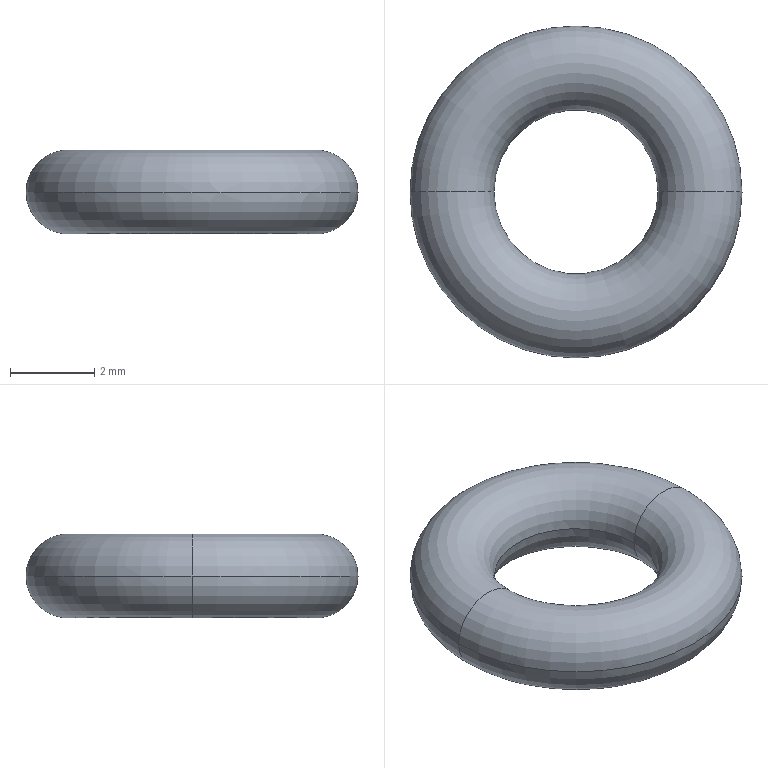Part | STEP file | ZXW722-L-79-3 | 1 solid | 4 faces | box 7.9 x 7.9 x 2 mm | volume 58.231 mm3 | torus 4
STEP:
#1=CARTESIAN_POINT('',(0.,0.,0.));
#2=DIRECTION('',(0.,0.,1.));
#3=DIRECTION('',(1.,0.,0.));
#4=AXIS2_PLACEMENT_3D('',#1,#2,#3);
#5=CARTESIAN_POINT('',(1.95,0.,-1.));
#6=VERTEX_POINT('',#5);
#7=CARTESIAN_POINT('',(3.95,0.,-1.));
#8=VERTEX_POINT('',#7);
#9=CARTESIAN_POINT('',(2.95,0.,-1.));
#10=DIRECTION('',(0.,-1.,0.));
#11=DIRECTION('',(-1.,0.,0.));
#12=AXIS2_PLACEMENT_3D('',#9,#10,#11);
#13=CIRCLE('',#12,1.);
#14=EDGE_CURVE('',#6,#8,#13,.T.);
#15=ORIENTED_EDGE('',*,*,#14,.T.);
#16=CARTESIAN_POINT('',(-3.95,0.,-1.));
#17=VERTEX_POINT('',#16);
#18=CARTESIAN_POINT('',(0.,0.,-1.));
#19=DIRECTION('',(0.,0.,-1.));
#20=DIRECTION('',(-1.,0.,0.));
#21=AXIS2_PLACEMENT_3D('',#18,#19,#20);
#22=CIRCLE('',#21,3.95);
#23=EDGE_CURVE('',#17,#8,#22,.T.);
#24=ORIENTED_EDGE('',*,*,#23,.F.);
#25=CARTESIAN_POINT('',(-1.95,0.,-1.));
#26=VERTEX_POINT('',#25);
#27=CARTESIAN_POINT('',(-2.95,0.,-1.));
#28=DIRECTION('',(0.,1.,0.));
#29=DIRECTION('',(1.,0.,0.));
#30=AXIS2_PLACEMENT_3D('',#27,#28,#29);
#31=CIRCLE('',#30,1.);
#32=EDGE_CURVE('',#26,#17,#31,.T.);
#33=ORIENTED_EDGE('',*,*,#32,.F.);
#34=CARTESIAN_POINT('',(0.,0.,-1.));
#35=DIRECTION('',(0.,0.,-1.));
#36=DIRECTION('',(-1.,0.,0.));
#37=AXIS2_PLACEMENT_3D('',#34,#35,#36);
#38=CIRCLE('',#37,1.95);
#39=EDGE_CURVE('',#26,#6,#38,.T.);
#40=ORIENTED_EDGE('',*,*,#39,.T.);
#41=EDGE_LOOP('',(#15,#24,#33,#40));
#42=FACE_OUTER_BOUND('',#41,.F.);
#43=CARTESIAN_POINT('',(0.,0.,-1.));
#44=DIRECTION('',(0.,0.,1.));
#45=DIRECTION('',(-1.,0.,0.));
#46=AXIS2_PLACEMENT_3D('',#43,#44,#45);
#47=TOROIDAL_SURFACE('',#46,2.95,1.);
#48=ADVANCED_FACE('',(#42),#47,.T.);
#49=ORIENTED_EDGE('',*,*,#14,.F.);
#50=CARTESIAN_POINT('',(0.,0.,-1.));
#51=DIRECTION('',(0.,0.,1.));
#52=DIRECTION('',(-1.,0.,0.));
#53=AXIS2_PLACEMENT_3D('',#50,#51,#52);
#54=CIRCLE('',#53,1.95);
#55=EDGE_CURVE('',#26,#6,#54,.T.);
#56=ORIENTED_EDGE('',*,*,#55,.F.);
#57=ORIENTED_EDGE('',*,*,#32,.T.);
#58=CARTESIAN_POINT('',(0.,0.,-1.));
#59=DIRECTION('',(0.,0.,1.));
#60=DIRECTION('',(-1.,0.,0.));
#61=AXIS2_PLACEMENT_3D('',#58,#59,#60);
#62=CIRCLE('',#61,3.95);
#63=EDGE_CURVE('',#17,#8,#62,.T.);
#64=ORIENTED_EDGE('',*,*,#63,.T.);
#65=EDGE_LOOP('',(#49,#56,#57,#64));
#66=FACE_OUTER_BOUND('',#65,.F.);
#67=CARTESIAN_POINT('',(0.,0.,-1.));
#68=DIRECTION('',(0.,0.,1.));
#69=DIRECTION('',(-1.,0.,0.));
#70=AXIS2_PLACEMENT_3D('',#67,#68,#69);
#71=TOROIDAL_SURFACE('',#70,2.95,1.);
#72=ADVANCED_FACE('',(#66),#71,.T.);
#73=CARTESIAN_POINT('',(2.95,0.,-1.));
#74=DIRECTION('',(0.,-1.,0.));
#75=DIRECTION('',(1.,0.,0.));
#76=AXIS2_PLACEMENT_3D('',#73,#74,#75);
#77=CIRCLE('',#76,1.);
#78=EDGE_CURVE('',#8,#6,#77,.T.);
#79=ORIENTED_EDGE('',*,*,#78,.F.);
#80=ORIENTED_EDGE('',*,*,#63,.F.);
#81=CARTESIAN_POINT('',(-2.95,0.,-1.));
#82=DIRECTION('',(0.,1.,0.));
#83=DIRECTION('',(-1.,0.,0.));
#84=AXIS2_PLACEMENT_3D('',#81,#82,#83);
#85=CIRCLE('',#84,1.);
#86=EDGE_CURVE('',#17,#26,#85,.T.);
#87=ORIENTED_EDGE('',*,*,#86,.T.);
#88=ORIENTED_EDGE('',*,*,#55,.T.);
#89=EDGE_LOOP('',(#79,#80,#87,#88));
#90=FACE_OUTER_BOUND('',#89,.F.);
#91=CARTESIAN_POINT('',(0.,0.,-1.));
#92=DIRECTION('',(0.,0.,1.));
#93=DIRECTION('',(-1.,0.,0.));
#94=AXIS2_PLACEMENT_3D('',#91,#92,#93);
#95=TOROIDAL_SURFACE('',#94,2.95,1.);
#96=ADVANCED_FACE('',(#90),#95,.T.);
#97=ORIENTED_EDGE('',*,*,#78,.T.);
#98=ORIENTED_EDGE('',*,*,#39,.F.);
#99=ORIENTED_EDGE('',*,*,#86,.F.);
#100=ORIENTED_EDGE('',*,*,#23,.T.);
#101=EDGE_LOOP('',(#97,#98,#99,#100));
#102=FACE_OUTER_BOUND('',#101,.F.);
#103=CARTESIAN_POINT('',(0.,0.,-1.));
#104=DIRECTION('',(0.,0.,1.));
#105=DIRECTION('',(-1.,0.,0.));
#106=AXIS2_PLACEMENT_3D('',#103,#104,#105);
#107=TOROIDAL_SURFACE('',#106,2.95,1.);
#108=ADVANCED_FACE('',(#102),#107,.T.);
#109=CLOSED_SHELL('',(#48,#72,#96,#108));
#110=MANIFOLD_SOLID_BREP('',#109);
#111=(LENGTH_UNIT()NAMED_UNIT(*)SI_UNIT(.MILLI.,.METRE.));
#112=UNCERTAINTY_MEASURE_WITH_UNIT(LENGTH_MEASURE(0.001135),#111,'','');
#113=(NAMED_UNIT(*)PLANE_ANGLE_UNIT()SI_UNIT($,.RADIAN.));
#114=PLANE_ANGLE_MEASURE_WITH_UNIT(PLANE_ANGLE_MEASURE(0.01745),#113);
#115=(CONVERSION_BASED_UNIT('DEGREE',#114)NAMED_UNIT(*)PLANE_ANGLE_UNIT());
#116=(NAMED_UNIT(*)SI_UNIT($,.STERADIAN.)SOLID_ANGLE_UNIT());
#117=(GEOMETRIC_REPRESENTATION_CONTEXT(3)GLOBAL_UNCERTAINTY_ASSIGNED_CONTEXT((#112))GLOBAL_UNIT_ASSIGNED_CONTEXT((#111,#115,#116))REPRESENTATION_CONTEXT('',''));
#118=ADVANCED_BREP_SHAPE_REPRESENTATION('',(#4,#110),#117);